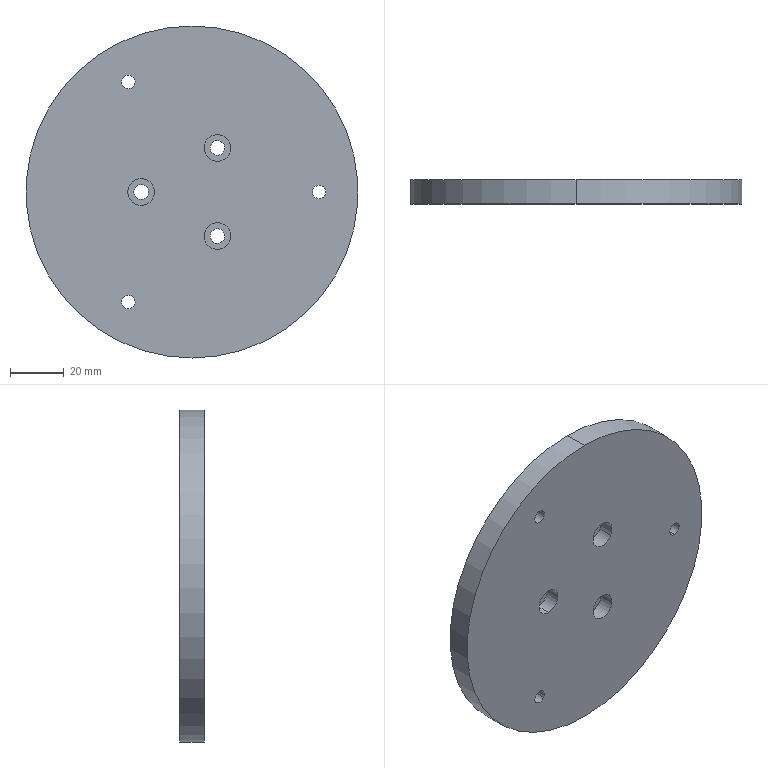Part | STEP file | PN_0061 fixing block | 1 solid | 28 faces | box 124 x 9 x 124 mm | volume 101363 mm3 | cylinder 22 | plane 6 | commonest cylinder face diameters 5 x6 5.5 x6 10 x6 48 x2 124 x2